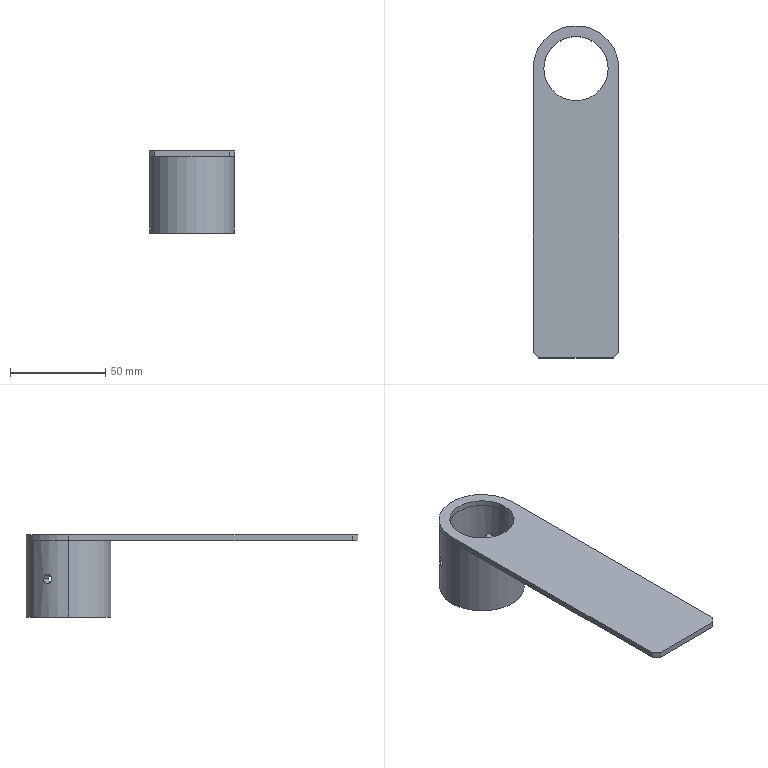Part | SolidWorks | features HoleWzd 3, 3DProfileFeature 1, Chamfer 1, Extrusion 1, ICE 1 | 2 solids | 20 faces | box 45 x 174.185 x 43 mm | volume 46480 mm3 | cylinder 11 | plane 9 | commonest cylinder face diameters 5 x4 33.7 x4 44.5 x2 45 x1
STEP:
#1=CARTESIAN_POINT('',(16.85,0.,20.));
#2=VERTEX_POINT('',#1);
#3=CARTESIAN_POINT('',(-16.85,0.,20.));
#4=VERTEX_POINT('',#3);
#5=CARTESIAN_POINT('',(0.,0.,20.));
#6=DIRECTION('',(0.,0.,-1.));
#7=DIRECTION('',(-1.,0.,0.));
#8=AXIS2_PLACEMENT_3D('',#5,#6,#7);
#9=CIRCLE('',#8,16.85);
#10=EDGE_CURVE('',#2,#4,#9,.T.);
#11=ORIENTED_EDGE('',*,*,#10,.T.);
#12=CARTESIAN_POINT('',(-16.85,0.,23.));
#13=VERTEX_POINT('',#12);
#14=CARTESIAN_POINT('',(-16.85,0.,23.));
#15=DIRECTION('',(0.,0.,1.));
#16=VECTOR('',#15,1000.);
#17=LINE('',#14,#16);
#18=EDGE_CURVE('',#4,#13,#17,.T.);
#19=ORIENTED_EDGE('',*,*,#18,.T.);
#20=CARTESIAN_POINT('',(16.85,0.,23.));
#21=VERTEX_POINT('',#20);
#22=CARTESIAN_POINT('',(0.,0.,23.));
#23=DIRECTION('',(0.,0.,1.));
#24=DIRECTION('',(1.,0.,0.));
#25=AXIS2_PLACEMENT_3D('',#22,#23,#24);
#26=CIRCLE('',#25,16.85);
#27=EDGE_CURVE('',#13,#21,#26,.T.);
#28=ORIENTED_EDGE('',*,*,#27,.T.);
#29=CARTESIAN_POINT('',(16.85,0.,23.));
#30=DIRECTION('',(0.,0.,1.));
#31=VECTOR('',#30,1000.);
#32=LINE('',#29,#31);
#33=EDGE_CURVE('',#2,#21,#32,.T.);
#34=ORIENTED_EDGE('',*,*,#33,.F.);
#35=EDGE_LOOP('',(#11,#19,#28,#34));
#36=FACE_OUTER_BOUND('',#35,.T.);
#37=CARTESIAN_POINT('',(0.,0.,23.));
#38=DIRECTION('',(0.,0.,1.));
#39=DIRECTION('',(1.,0.,0.));
#40=AXIS2_PLACEMENT_3D('',#37,#38,#39);
#41=CYLINDRICAL_SURFACE('',#40,16.85);
#42=ADVANCED_FACE('',(#36),#41,.F.);
#43=CARTESIAN_POINT('',(-22.5,0.,20.));
#44=VERTEX_POINT('',#43);
#45=CARTESIAN_POINT('',(22.5,0.,20.));
#46=VERTEX_POINT('',#45);
#47=CARTESIAN_POINT('',(0.,0.,20.));
#48=DIRECTION('',(0.,0.,-1.));
#49=DIRECTION('',(-1.,0.,0.));
#50=AXIS2_PLACEMENT_3D('',#47,#48,#49);
#51=CIRCLE('',#50,22.5);
#52=EDGE_CURVE('',#44,#46,#51,.T.);
#53=ORIENTED_EDGE('',*,*,#52,.F.);
#54=CARTESIAN_POINT('',(-22.5,0.,23.));
#55=VERTEX_POINT('',#54);
#56=CARTESIAN_POINT('',(-22.5,0.,23.));
#57=DIRECTION('',(0.,0.,-1.));
#58=VECTOR('',#57,1000.);
#59=LINE('',#56,#58);
#60=EDGE_CURVE('',#55,#44,#59,.T.);
#61=ORIENTED_EDGE('',*,*,#60,.F.);
#62=CARTESIAN_POINT('',(22.5,0.,23.));
#63=VERTEX_POINT('',#62);
#64=CARTESIAN_POINT('',(0.,0.,23.));
#65=DIRECTION('',(0.,0.,-1.));
#66=DIRECTION('',(-1.,0.,0.));
#67=AXIS2_PLACEMENT_3D('',#64,#65,#66);
#68=CIRCLE('',#67,22.5);
#69=EDGE_CURVE('',#55,#63,#68,.T.);
#70=ORIENTED_EDGE('',*,*,#69,.T.);
#71=CARTESIAN_POINT('',(22.5,0.,23.));
#72=DIRECTION('',(0.,0.,-1.));
#73=VECTOR('',#72,1000.);
#74=LINE('',#71,#73);
#75=EDGE_CURVE('',#63,#46,#74,.T.);
#76=ORIENTED_EDGE('',*,*,#75,.T.);
#77=EDGE_LOOP('',(#53,#61,#70,#76));
#78=FACE_OUTER_BOUND('',#77,.T.);
#79=CARTESIAN_POINT('',(0.,0.,23.));
#80=DIRECTION('',(0.,0.,-1.));
#81=DIRECTION('',(-1.,0.,0.));
#82=AXIS2_PLACEMENT_3D('',#79,#80,#81);
#83=CYLINDRICAL_SURFACE('',#82,22.5);
#84=ADVANCED_FACE('',(#78),#83,.T.);
#85=CARTESIAN_POINT('',(-22.5,-148.685,20.));
#86=VERTEX_POINT('',#85);
#87=CARTESIAN_POINT('',(-22.5,-151.685,20.));
#88=DIRECTION('',(0.,1.,0.));
#89=VECTOR('',#88,1000.);
#90=LINE('',#87,#89);
#91=EDGE_CURVE('',#86,#44,#90,.T.);
#92=ORIENTED_EDGE('',*,*,#91,.F.);
#93=CARTESIAN_POINT('',(-22.5,-148.685,23.));
#94=VERTEX_POINT('',#93);
#95=CARTESIAN_POINT('',(-22.5,-148.685,23.));
#96=DIRECTION('',(0.,0.,1.));
#97=VECTOR('',#96,1000.);
#98=LINE('',#95,#97);
#99=EDGE_CURVE('',#86,#94,#98,.T.);
#100=ORIENTED_EDGE('',*,*,#99,.T.);
#101=CARTESIAN_POINT('',(-22.5,-151.685,23.));
#102=DIRECTION('',(0.,1.,0.));
#103=VECTOR('',#102,1000.);
#104=LINE('',#101,#103);
#105=EDGE_CURVE('',#94,#55,#104,.T.);
#106=ORIENTED_EDGE('',*,*,#105,.T.);
#107=ORIENTED_EDGE('',*,*,#60,.T.);
#108=EDGE_LOOP('',(#92,#100,#106,#107));
#109=FACE_OUTER_BOUND('',#108,.T.);
#110=CARTESIAN_POINT('',(-22.5,-151.685,23.));
#111=DIRECTION('',(-1.,0.,0.));
#112=DIRECTION('',(0.,-1.,0.));
#113=AXIS2_PLACEMENT_3D('',#110,#111,#112);
#114=PLANE('',#113);
#115=ADVANCED_FACE('',(#109),#114,.T.);
#116=CARTESIAN_POINT('',(19.5,-151.685,23.));
#117=VERTEX_POINT('',#116);
#118=CARTESIAN_POINT('',(-19.5,-151.685,23.));
#119=VERTEX_POINT('',#118);
#120=CARTESIAN_POINT('',(22.5,-151.685,23.));
#121=DIRECTION('',(-1.,0.,0.));
#122=VECTOR('',#121,1000.);
#123=LINE('',#120,#122);
#124=EDGE_CURVE('',#117,#119,#123,.T.);
#125=ORIENTED_EDGE('',*,*,#124,.T.);
#126=CARTESIAN_POINT('',(-19.5,-151.685,20.));
#127=VERTEX_POINT('',#126);
#128=CARTESIAN_POINT('',(-19.5,-151.685,23.));
#129=DIRECTION('',(0.,0.,-1.));
#130=VECTOR('',#129,1000.);
#131=LINE('',#128,#130);
#132=EDGE_CURVE('',#119,#127,#131,.T.);
#133=ORIENTED_EDGE('',*,*,#132,.T.);
#134=CARTESIAN_POINT('',(19.5,-151.685,20.));
#135=VERTEX_POINT('',#134);
#136=CARTESIAN_POINT('',(22.5,-151.685,20.));
#137=DIRECTION('',(-1.,0.,0.));
#138=VECTOR('',#137,1000.);
#139=LINE('',#136,#138);
#140=EDGE_CURVE('',#135,#127,#139,.T.);
#141=ORIENTED_EDGE('',*,*,#140,.F.);
#142=CARTESIAN_POINT('',(19.5,-151.685,23.));
#143=DIRECTION('',(0.,0.,1.));
#144=VECTOR('',#143,1000.);
#145=LINE('',#142,#144);
#146=EDGE_CURVE('',#135,#117,#145,.T.);
#147=ORIENTED_EDGE('',*,*,#146,.T.);
#148=EDGE_LOOP('',(#125,#133,#141,#147));
#149=FACE_OUTER_BOUND('',#148,.T.);
#150=CARTESIAN_POINT('',(22.5,-151.685,23.));
#151=DIRECTION('',(0.,-1.,0.));
#152=DIRECTION('',(0.,0.,-1.));
#153=AXIS2_PLACEMENT_3D('',#150,#151,#152);
#154=PLANE('',#153);
#155=ADVANCED_FACE('',(#149),#154,.T.);
#156=CARTESIAN_POINT('',(22.5,-148.685,23.));
#157=VERTEX_POINT('',#156);
#158=CARTESIAN_POINT('',(22.5,0.,23.));
#159=DIRECTION('',(0.,-1.,0.));
#160=VECTOR('',#159,1000.);
#161=LINE('',#158,#160);
#162=EDGE_CURVE('',#63,#157,#161,.T.);
#163=ORIENTED_EDGE('',*,*,#162,.T.);
#164=CARTESIAN_POINT('',(22.5,-148.685,20.));
#165=VERTEX_POINT('',#164);
#166=CARTESIAN_POINT('',(22.5,-148.685,23.));
#167=DIRECTION('',(0.,0.,-1.));
#168=VECTOR('',#167,1000.);
#169=LINE('',#166,#168);
#170=EDGE_CURVE('',#157,#165,#169,.T.);
#171=ORIENTED_EDGE('',*,*,#170,.T.);
#172=CARTESIAN_POINT('',(22.5,0.,20.));
#173=DIRECTION('',(0.,-1.,0.));
#174=VECTOR('',#173,1000.);
#175=LINE('',#172,#174);
#176=EDGE_CURVE('',#46,#165,#175,.T.);
#177=ORIENTED_EDGE('',*,*,#176,.F.);
#178=ORIENTED_EDGE('',*,*,#75,.F.);
#179=EDGE_LOOP('',(#163,#171,#177,#178));
#180=FACE_OUTER_BOUND('',#179,.T.);
#181=CARTESIAN_POINT('',(22.5,0.,23.));
#182=DIRECTION('',(1.,0.,0.));
#183=DIRECTION('',(0.,1.,0.));
#184=AXIS2_PLACEMENT_3D('',#181,#182,#183);
#185=PLANE('',#184);
#186=ADVANCED_FACE('',(#180),#185,.T.);
#187=CARTESIAN_POINT('',(0.,0.,23.));
#188=DIRECTION('',(0.,0.,1.));
#189=DIRECTION('',(1.,0.,0.));
#190=AXIS2_PLACEMENT_3D('',#187,#188,#189);
#191=CIRCLE('',#190,16.85);
#192=EDGE_CURVE('',#21,#13,#191,.T.);
#193=ORIENTED_EDGE('',*,*,#192,.F.);
#194=ORIENTED_EDGE('',*,*,#27,.F.);
#195=EDGE_LOOP('',(#193,#194));
#196=FACE_BOUND('',#195,.T.);
#197=ORIENTED_EDGE('',*,*,#105,.F.);
#198=CARTESIAN_POINT('',(-19.5,-151.685,23.));
#199=DIRECTION('',(0.7071,-0.7071,0.));
#200=VECTOR('',#199,1000.);
#201=LINE('',#198,#200);
#202=EDGE_CURVE('',#94,#119,#201,.T.);
#203=ORIENTED_EDGE('',*,*,#202,.T.);
#204=ORIENTED_EDGE('',*,*,#124,.F.);
#205=CARTESIAN_POINT('',(22.5,-148.685,23.));
#206=DIRECTION('',(0.7071,0.7071,0.));
#207=VECTOR('',#206,1000.);
#208=LINE('',#205,#207);
#209=EDGE_CURVE('',#117,#157,#208,.T.);
#210=ORIENTED_EDGE('',*,*,#209,.T.);
#211=ORIENTED_EDGE('',*,*,#162,.F.);
#212=ORIENTED_EDGE('',*,*,#69,.F.);
#213=EDGE_LOOP('',(#197,#203,#204,#210,#211,#212));
#214=FACE_OUTER_BOUND('',#213,.T.);
#215=CARTESIAN_POINT('',(0.,0.,23.));
#216=DIRECTION('',(0.,0.,-1.));
#217=DIRECTION('',(-1.,0.,0.));
#218=AXIS2_PLACEMENT_3D('',#215,#216,#217);
#219=PLANE('',#218);
#220=ADVANCED_FACE('',(#196,#214),#219,.F.);
#221=ORIENTED_EDGE('',*,*,#10,.F.);
#222=CARTESIAN_POINT('',(0.,0.,20.));
#223=DIRECTION('',(0.,0.,-1.));
#224=DIRECTION('',(-1.,0.,0.));
#225=AXIS2_PLACEMENT_3D('',#222,#223,#224);
#226=CIRCLE('',#225,16.85);
#227=EDGE_CURVE('',#4,#2,#226,.T.);
#228=ORIENTED_EDGE('',*,*,#227,.F.);
#229=EDGE_LOOP('',(#221,#228));
#230=FACE_BOUND('',#229,.T.);
#231=ORIENTED_EDGE('',*,*,#140,.T.);
#232=CARTESIAN_POINT('',(-85.593,-85.593,20.));
#233=DIRECTION('',(-0.7071,0.7071,0.));
#234=VECTOR('',#233,1000.);
#235=LINE('',#232,#234);
#236=EDGE_CURVE('',#127,#86,#235,.T.);
#237=ORIENTED_EDGE('',*,*,#236,.T.);
#238=ORIENTED_EDGE('',*,*,#91,.T.);
#239=ORIENTED_EDGE('',*,*,#52,.T.);
#240=ORIENTED_EDGE('',*,*,#176,.T.);
#241=CARTESIAN_POINT('',(85.593,-85.593,20.));
#242=DIRECTION('',(-0.7071,-0.7071,0.));
#243=VECTOR('',#242,1000.);
#244=LINE('',#241,#243);
#245=EDGE_CURVE('',#165,#135,#244,.T.);
#246=ORIENTED_EDGE('',*,*,#245,.T.);
#247=EDGE_LOOP('',(#231,#237,#238,#239,#240,#246));
#248=FACE_OUTER_BOUND('',#247,.T.);
#249=CARTESIAN_POINT('',(0.,0.,20.));
#250=DIRECTION('',(0.,0.,-1.));
#251=DIRECTION('',(-1.,0.,0.));
#252=AXIS2_PLACEMENT_3D('',#249,#250,#251);
#253=PLANE('',#252);
#254=ADVANCED_FACE('',(#230,#248),#253,.T.);
#255=ORIENTED_EDGE('',*,*,#18,.F.);
#256=ORIENTED_EDGE('',*,*,#227,.T.);
#257=ORIENTED_EDGE('',*,*,#33,.T.);
#258=ORIENTED_EDGE('',*,*,#192,.T.);
#259=EDGE_LOOP('',(#255,#256,#257,#258));
#260=FACE_OUTER_BOUND('',#259,.T.);
#261=CARTESIAN_POINT('',(0.,0.,23.));
#262=DIRECTION('',(0.,0.,1.));
#263=DIRECTION('',(1.,0.,0.));
#264=AXIS2_PLACEMENT_3D('',#261,#262,#263);
#265=CYLINDRICAL_SURFACE('',#264,16.85);
#266=ADVANCED_FACE('',(#260),#265,.F.);
#267=ORIENTED_EDGE('',*,*,#202,.F.);
#268=ORIENTED_EDGE('',*,*,#99,.F.);
#269=ORIENTED_EDGE('',*,*,#236,.F.);
#270=ORIENTED_EDGE('',*,*,#132,.F.);
#271=EDGE_LOOP('',(#267,#268,#269,#270));
#272=FACE_OUTER_BOUND('',#271,.T.);
#273=CARTESIAN_POINT('',(-19.5,-151.685,23.));
#274=DIRECTION('',(0.7071,0.7071,0.));
#275=DIRECTION('',(0.,0.,-1.));
#276=AXIS2_PLACEMENT_3D('',#273,#274,#275);
#277=PLANE('',#276);
#278=ADVANCED_FACE('',(#272),#277,.F.);
#279=ORIENTED_EDGE('',*,*,#209,.F.);
#280=ORIENTED_EDGE('',*,*,#146,.F.);
#281=ORIENTED_EDGE('',*,*,#245,.F.);
#282=ORIENTED_EDGE('',*,*,#170,.F.);
#283=EDGE_LOOP('',(#279,#280,#281,#282));
#284=FACE_OUTER_BOUND('',#283,.T.);
#285=CARTESIAN_POINT('',(22.5,-148.685,23.));
#286=DIRECTION('',(-0.7071,0.7071,0.));
#287=DIRECTION('',(0.,0.,-1.));
#288=AXIS2_PLACEMENT_3D('',#285,#286,#287);
#289=PLANE('',#288);
#290=ADVANCED_FACE('',(#284),#289,.F.);
#291=CLOSED_SHELL('',(#42,#84,#115,#155,#186,#220,#254,#266,#278,#290));
#292=MANIFOLD_SOLID_BREP('',#291);
#293=CARTESIAN_POINT('',(17.897,13.22,0.));
#294=VERTEX_POINT('',#293);
#295=CARTESIAN_POINT('',(20.397,8.889,0.));
#296=VERTEX_POINT('',#295);
#297=CARTESIAN_POINT('',(17.897,13.22,0.));
#298=CARTESIAN_POINT('',(17.897,13.22,-0.1632));
#299=CARTESIAN_POINT('',(17.907,13.207,-0.3255));
#300=CARTESIAN_POINT('',(17.945,13.155,-0.6482));
#301=CARTESIAN_POINT('',(17.973,13.116,-0.8059));
#302=CARTESIAN_POINT('',(18.047,13.015,-1.107));
#303=CARTESIAN_POINT('',(18.092,12.951,-1.252));
#304=CARTESIAN_POINT('',(18.198,12.802,-1.525));
#305=CARTESIAN_POINT('',(18.258,12.717,-1.651));
#306=CARTESIAN_POINT('',(18.389,12.527,-1.882));
#307=CARTESIAN_POINT('',(18.461,12.42,-1.987));
#308=CARTESIAN_POINT('',(18.612,12.193,-2.169));
#309=CARTESIAN_POINT('',(18.69,12.073,-2.246));
#310=CARTESIAN_POINT('',(18.853,11.818,-2.372));
#311=CARTESIAN_POINT('',(18.937,11.683,-2.42));
#312=CARTESIAN_POINT('',(19.103,11.409,-2.484));
#313=CARTESIAN_POINT('',(19.186,11.27,-2.5));
#314=CARTESIAN_POINT('',(19.351,10.984,-2.5));
#315=CARTESIAN_POINT('',(19.43,10.842,-2.484));
#316=CARTESIAN_POINT('',(19.584,10.561,-2.421));
#317=CARTESIAN_POINT('',(19.659,10.421,-2.373));
#318=CARTESIAN_POINT('',(19.799,10.153,-2.247));
#319=CARTESIAN_POINT('',(19.864,10.024,-2.171));
#320=CARTESIAN_POINT('',(19.986,9.78,-1.99));
#321=CARTESIAN_POINT('',(20.042,9.664,-1.884));
#322=CARTESIAN_POINT('',(20.141,9.456,-1.654));
#323=CARTESIAN_POINT('',(20.185,9.361,-1.528));
#324=CARTESIAN_POINT('',(20.262,9.194,-1.255));
#325=CARTESIAN_POINT('',(20.294,9.123,-1.11));
#326=CARTESIAN_POINT('',(20.371,8.951,-0.659));
#327=CARTESIAN_POINT('',(20.397,8.889,-0.3306));
#328=CARTESIAN_POINT('',(20.397,8.889,0.));
#329=B_SPLINE_CURVE_WITH_KNOTS('',3,(#297,#298,#299,#300,#301,#302,#303,#304,#305,#306,#307,#308,#309,#310,#311,#312,#313,#314,#315,#316,#317,#318,#319,#320,#321,#322,#323,#324,#325,#326,#327,#328),.UNSPECIFIED.,.F.,.F.,(4,2,2,2,2,2,2,2,2,2,2,2,2,2,2,4),(0.007822,0.008311,0.0088,0.009289,0.009777,0.01027,0.01075,0.01124,0.01173,0.01222,0.01271,0.0132,0.01369,0.01418,0.01467,0.01564),.UNSPECIFIED.);
#330=EDGE_CURVE('',#294,#296,#329,.T.);
#331=ORIENTED_EDGE('',*,*,#330,.F.);
#332=CARTESIAN_POINT('',(13.181,10.497,0.));
#333=VERTEX_POINT('',#332);
#334=CARTESIAN_POINT('',(13.181,10.497,0.));
#335=DIRECTION('',(-0.866,-0.5,0.));
#336=VECTOR('',#335,1000.);
#337=LINE('',#334,#336);
#338=EDGE_CURVE('',#294,#333,#337,.T.);
#339=ORIENTED_EDGE('',*,*,#338,.T.);
#340=CARTESIAN_POINT('',(15.681,6.167,0.));
#341=VERTEX_POINT('',#340);
#342=CARTESIAN_POINT('',(15.681,6.167,0.));
#343=CARTESIAN_POINT('',(15.681,6.167,-0.1654));
#344=CARTESIAN_POINT('',(15.675,6.182,-0.328));
#345=CARTESIAN_POINT('',(15.651,6.242,-0.6479));
#346=CARTESIAN_POINT('',(15.633,6.287,-0.8068));
#347=CARTESIAN_POINT('',(15.586,6.404,-1.109));
#348=CARTESIAN_POINT('',(15.556,6.476,-1.253));
#349=CARTESIAN_POINT('',(15.485,6.645,-1.525));
#350=CARTESIAN_POINT('',(15.443,6.742,-1.653));
#351=CARTESIAN_POINT('',(15.349,6.954,-1.883));
#352=CARTESIAN_POINT('',(15.296,7.069,-1.987));
#353=CARTESIAN_POINT('',(15.179,7.317,-2.169));
#354=CARTESIAN_POINT('',(15.116,7.447,-2.247));
#355=CARTESIAN_POINT('',(14.98,7.717,-2.372));
#356=CARTESIAN_POINT('',(14.907,7.857,-2.42));
#357=CARTESIAN_POINT('',(14.754,8.141,-2.484));
#358=CARTESIAN_POINT('',(14.675,8.283,-2.5));
#359=CARTESIAN_POINT('',(14.511,8.566,-2.5));
#360=CARTESIAN_POINT('',(14.426,8.708,-2.484));
#361=CARTESIAN_POINT('',(14.258,8.981,-2.42));
#362=CARTESIAN_POINT('',(14.174,9.113,-2.372));
#363=CARTESIAN_POINT('',(14.008,9.367,-2.247));
#364=CARTESIAN_POINT('',(13.925,9.488,-2.169));
#365=CARTESIAN_POINT('',(13.771,9.711,-1.988));
#366=CARTESIAN_POINT('',(13.697,9.815,-1.884));
#367=CARTESIAN_POINT('',(13.559,10.004,-1.651));
#368=CARTESIAN_POINT('',(13.497,10.087,-1.525));
#369=CARTESIAN_POINT('',(13.387,10.233,-1.255));
#370=CARTESIAN_POINT('',(13.339,10.296,-1.108));
#371=CARTESIAN_POINT('',(13.261,10.396,-0.8059));
#372=CARTESIAN_POINT('',(13.232,10.433,-0.65));
#373=CARTESIAN_POINT('',(13.191,10.484,-0.3291));
#374=CARTESIAN_POINT('',(13.181,10.497,-0.1633));
#375=CARTESIAN_POINT('',(13.181,10.497,0.));
#376=B_SPLINE_CURVE_WITH_KNOTS('',3,(#342,#343,#344,#345,#346,#347,#348,#349,#350,#351,#352,#353,#354,#355,#356,#357,#358,#359,#360,#361,#362,#363,#364,#365,#366,#367,#368,#369,#370,#371,#372,#373,#374,#375),.UNSPECIFIED.,.F.,.F.,(4,2,2,2,2,2,2,2,2,2,2,2,2,2,2,2,4),(0.,0.0004892,0.0009784,0.001468,0.001957,0.002446,0.002935,0.003424,0.003913,0.004403,0.004892,0.005381,0.00587,0.006359,0.006849,0.007338,0.007827),.UNSPECIFIED.);
#377=EDGE_CURVE('',#341,#333,#376,.T.);
#378=ORIENTED_EDGE('',*,*,#377,.F.);
#379=CARTESIAN_POINT('',(15.681,6.167,0.));
#380=DIRECTION('',(-0.866,-0.5,0.));
#381=VECTOR('',#380,1000.);
#382=LINE('',#379,#381);
#383=EDGE_CURVE('',#296,#341,#382,.T.);
#384=ORIENTED_EDGE('',*,*,#383,.F.);
#385=EDGE_LOOP('',(#331,#339,#378,#384));
#386=FACE_OUTER_BOUND('',#385,.T.);
#387=CARTESIAN_POINT('',(14.431,8.332,0.));
#388=DIRECTION('',(-0.866,-0.5,0.));
#389=DIRECTION('',(0.5,-0.866,0.));
#390=AXIS2_PLACEMENT_3D('',#387,#388,#389);
#391=CYLINDRICAL_SURFACE('',#390,2.5);
#392=ADVANCED_FACE('',(#386),#391,.F.);
#393=CARTESIAN_POINT('',(-13.181,10.497,0.));
#394=VERTEX_POINT('',#393);
#395=CARTESIAN_POINT('',(-15.681,6.167,0.));
#396=VERTEX_POINT('',#395);
#397=CARTESIAN_POINT('',(-13.181,10.497,0.));
#398=CARTESIAN_POINT('',(-13.181,10.497,-0.3265));
#399=CARTESIAN_POINT('',(-13.223,10.445,-0.6558));
#400=CARTESIAN_POINT('',(-13.339,10.296,-1.107));
#401=CARTESIAN_POINT('',(-13.386,10.234,-1.253));
#402=CARTESIAN_POINT('',(-13.497,10.087,-1.526));
#403=CARTESIAN_POINT('',(-13.559,10.004,-1.651));
#404=CARTESIAN_POINT('',(-13.696,9.817,-1.882));
#405=CARTESIAN_POINT('',(-13.77,9.712,-1.987));
#406=CARTESIAN_POINT('',(-13.925,9.488,-2.169));
#407=CARTESIAN_POINT('',(-14.006,9.369,-2.246));
#408=CARTESIAN_POINT('',(-14.172,9.115,-2.371));
#409=CARTESIAN_POINT('',(-14.258,8.982,-2.42));
#410=CARTESIAN_POINT('',(-14.425,8.709,-2.484));
#411=CARTESIAN_POINT('',(-14.509,8.569,-2.5));
#412=CARTESIAN_POINT('',(-14.674,8.283,-2.5));
#413=CARTESIAN_POINT('',(-14.754,8.141,-2.484));
#414=CARTESIAN_POINT('',(-14.905,7.86,-2.421));
#415=CARTESIAN_POINT('',(-14.979,7.718,-2.372));
#416=CARTESIAN_POINT('',(-15.115,7.448,-2.247));
#417=CARTESIAN_POINT('',(-15.178,7.318,-2.171));
#418=CARTESIAN_POINT('',(-15.295,7.072,-1.989));
#419=CARTESIAN_POINT('',(-15.348,6.954,-1.884));
#420=CARTESIAN_POINT('',(-15.49,6.637,-1.539));
#421=CARTESIAN_POINT('',(-15.562,6.463,-1.261));
#422=CARTESIAN_POINT('',(-15.633,6.288,-0.8097));
#423=CARTESIAN_POINT('',(-15.651,6.243,-0.6518));
#424=CARTESIAN_POINT('',(-15.675,6.182,-0.3288));
#425=CARTESIAN_POINT('',(-15.681,6.167,-0.1654));
#426=CARTESIAN_POINT('',(-15.681,6.167,0.));
#427=B_SPLINE_CURVE_WITH_KNOTS('',3,(#397,#398,#399,#400,#401,#402,#403,#404,#405,#406,#407,#408,#409,#410,#411,#412,#413,#414,#415,#416,#417,#418,#419,#420,#421,#422,#423,#424,#425,#426),.UNSPECIFIED.,.F.,.F.,(4,2,2,2,2,2,2,2,2,2,2,2,2,2,4),(0.007827,0.008805,0.009294,0.009783,0.01027,0.01076,0.01125,0.01174,0.01223,0.01272,0.01321,0.0137,0.01467,0.01516,0.01565),.UNSPECIFIED.);
#428=EDGE_CURVE('',#394,#396,#427,.T.);
#429=ORIENTED_EDGE('',*,*,#428,.F.);
#430=CARTESIAN_POINT('',(-17.897,13.22,0.));
#431=VERTEX_POINT('',#430);
#432=CARTESIAN_POINT('',(-18.236,13.415,0.));
#433=DIRECTION('',(-0.866,0.5,0.));
#434=VECTOR('',#433,1000.);
#435=LINE('',#432,#434);
#436=EDGE_CURVE('',#394,#431,#435,.T.);
#437=ORIENTED_EDGE('',*,*,#436,.T.);
#438=CARTESIAN_POINT('',(-20.397,8.889,0.));
#439=VERTEX_POINT('',#438);
#440=CARTESIAN_POINT('',(-20.397,8.889,0.));
#441=CARTESIAN_POINT('',(-20.397,8.889,-0.1653));
#442=CARTESIAN_POINT('',(-20.391,8.904,-0.3279));
#443=CARTESIAN_POINT('',(-20.365,8.963,-0.6476));
#444=CARTESIAN_POINT('',(-20.345,9.007,-0.8064));
#445=CARTESIAN_POINT('',(-20.294,9.123,-1.109));
#446=CARTESIAN_POINT('',(-20.262,9.193,-1.253));
#447=CARTESIAN_POINT('',(-20.186,9.359,-1.524));
#448=CARTESIAN_POINT('',(-20.142,9.455,-1.653));
#449=CARTESIAN_POINT('',(-20.042,9.664,-1.883));
#450=CARTESIAN_POINT('',(-19.987,9.777,-1.987));
#451=CARTESIAN_POINT('',(-19.865,10.022,-2.17));
#452=CARTESIAN_POINT('',(-19.799,10.152,-2.247));
#453=CARTESIAN_POINT('',(-19.66,10.419,-2.372));
#454=CARTESIAN_POINT('',(-19.586,10.558,-2.42));
#455=CARTESIAN_POINT('',(-19.431,10.841,-2.484));
#456=CARTESIAN_POINT('',(-19.351,10.983,-2.5));
#457=CARTESIAN_POINT('',(-19.188,11.266,-2.5));
#458=CARTESIAN_POINT('',(-19.103,11.408,-2.484));
#459=CARTESIAN_POINT('',(-18.937,11.682,-2.42));
#460=CARTESIAN_POINT('',(-18.855,11.815,-2.373));
#461=CARTESIAN_POINT('',(-18.692,12.071,-2.247));
#462=CARTESIAN_POINT('',(-18.612,12.193,-2.169));
#463=CARTESIAN_POINT('',(-18.462,12.419,-1.988));
#464=CARTESIAN_POINT('',(-18.391,12.524,-1.885));
#465=CARTESIAN_POINT('',(-18.258,12.717,-1.651));
#466=CARTESIAN_POINT('',(-18.198,12.802,-1.525));
#467=CARTESIAN_POINT('',(-18.093,12.95,-1.254));
#468=CARTESIAN_POINT('',(-18.047,13.014,-1.108));
#469=CARTESIAN_POINT('',(-17.973,13.116,-0.8055));
#470=CARTESIAN_POINT('',(-17.945,13.155,-0.6497));
#471=CARTESIAN_POINT('',(-17.907,13.206,-0.329));
#472=CARTESIAN_POINT('',(-17.897,13.22,-0.1632));
#473=CARTESIAN_POINT('',(-17.897,13.22,0.));
#474=B_SPLINE_CURVE_WITH_KNOTS('',3,(#440,#441,#442,#443,#444,#445,#446,#447,#448,#449,#450,#451,#452,#453,#454,#455,#456,#457,#458,#459,#460,#461,#462,#463,#464,#465,#466,#467,#468,#469,#470,#471,#472,#473),.UNSPECIFIED.,.F.,.F.,(4,2,2,2,2,2,2,2,2,2,2,2,2,2,2,2,4),(0.,0.0004889,0.0009778,0.001467,0.001956,0.002444,0.002933,0.003422,0.003911,0.0044,0.004889,0.005378,0.005867,0.006356,0.006845,0.007333,0.007822),.UNSPECIFIED.);
#475=EDGE_CURVE('',#439,#431,#474,.T.);
#476=ORIENTED_EDGE('',*,*,#475,.F.);
#477=CARTESIAN_POINT('',(-20.736,9.085,0.));
#478=DIRECTION('',(-0.866,0.5,0.));
#479=VECTOR('',#478,1000.);
#480=LINE('',#477,#479);
#481=EDGE_CURVE('',#396,#439,#480,.T.);
#482=ORIENTED_EDGE('',*,*,#481,.F.);
#483=EDGE_LOOP('',(#429,#437,#476,#482));
#484=FACE_OUTER_BOUND('',#483,.T.);
#485=CARTESIAN_POINT('',(-19.486,11.25,0.));
#486=DIRECTION('',(-0.866,0.5,0.));
#487=DIRECTION('',(-0.5,-0.866,0.));
#488=AXIS2_PLACEMENT_3D('',#485,#486,#487);
#489=CYLINDRICAL_SURFACE('',#488,2.5);
#490=ADVANCED_FACE('',(#484),#489,.F.);
#491=CARTESIAN_POINT('',(-16.85,0.,-20.));
#492=VERTEX_POINT('',#491);
#493=CARTESIAN_POINT('',(16.85,0.,-20.));
#494=VERTEX_POINT('',#493);
#495=CARTESIAN_POINT('',(0.,0.,-20.));
#496=DIRECTION('',(0.,0.,1.));
#497=DIRECTION('',(1.,0.,0.));
#498=AXIS2_PLACEMENT_3D('',#495,#496,#497);
#499=CIRCLE('',#498,16.85);
#500=EDGE_CURVE('',#492,#494,#499,.T.);
#501=ORIENTED_EDGE('',*,*,#500,.F.);
#502=CARTESIAN_POINT('',(-16.85,0.,20.));
#503=VERTEX_POINT('',#502);
#504=CARTESIAN_POINT('',(-16.85,0.,23.));
#505=DIRECTION('',(0.,0.,1.));
#506=VECTOR('',#505,1000.);
#507=LINE('',#504,#506);
#508=EDGE_CURVE('',#492,#503,#507,.T.);
#509=ORIENTED_EDGE('',*,*,#508,.T.);
#510=CARTESIAN_POINT('',(16.85,0.,20.));
#511=VERTEX_POINT('',#510);
#512=CARTESIAN_POINT('',(0.,0.,20.));
#513=DIRECTION('',(0.,0.,-1.));
#514=DIRECTION('',(-1.,0.,0.));
#515=AXIS2_PLACEMENT_3D('',#512,#513,#514);
#516=CIRCLE('',#515,16.85);
#517=EDGE_CURVE('',#511,#503,#516,.T.);
#518=ORIENTED_EDGE('',*,*,#517,.F.);
#519=CARTESIAN_POINT('',(16.85,0.,23.));
#520=DIRECTION('',(0.,0.,1.));
#521=VECTOR('',#520,1000.);
#522=LINE('',#519,#521);
#523=EDGE_CURVE('',#494,#511,#522,.T.);
#524=ORIENTED_EDGE('',*,*,#523,.F.);
#525=EDGE_LOOP('',(#501,#509,#518,#524));
#526=FACE_OUTER_BOUND('',#525,.T.);
#527=CARTESIAN_POINT('',(0.,0.,23.));
#528=DIRECTION('',(0.,0.,1.));
#529=DIRECTION('',(1.,0.,0.));
#530=AXIS2_PLACEMENT_3D('',#527,#528,#529);
#531=CYLINDRICAL_SURFACE('',#530,16.85);
#532=ADVANCED_FACE('',(#526),#531,.F.);
#533=CARTESIAN_POINT('',(20.397,8.889,0.));
#534=CARTESIAN_POINT('',(20.397,8.889,0.1653));
#535=CARTESIAN_POINT('',(20.391,8.904,0.3279));
#536=CARTESIAN_POINT('',(20.365,8.963,0.6476));
#537=CARTESIAN_POINT('',(20.345,9.007,0.8064));
#538=CARTESIAN_POINT('',(20.294,9.123,1.109));
#539=CARTESIAN_POINT('',(20.262,9.193,1.253));
#540=CARTESIAN_POINT('',(20.186,9.359,1.524));
#541=CARTESIAN_POINT('',(20.142,9.455,1.653));
#542=CARTESIAN_POINT('',(20.042,9.664,1.883));
#543=CARTESIAN_POINT('',(19.987,9.777,1.987));
#544=CARTESIAN_POINT('',(19.865,10.022,2.17));
#545=CARTESIAN_POINT('',(19.799,10.152,2.247));
#546=CARTESIAN_POINT('',(19.66,10.419,2.372));
#547=CARTESIAN_POINT('',(19.586,10.558,2.42));
#548=CARTESIAN_POINT('',(19.431,10.841,2.484));
#549=CARTESIAN_POINT('',(19.351,10.983,2.5));
#550=CARTESIAN_POINT('',(19.188,11.266,2.5));
#551=CARTESIAN_POINT('',(19.103,11.408,2.484));
#552=CARTESIAN_POINT('',(18.937,11.682,2.42));
#553=CARTESIAN_POINT('',(18.855,11.815,2.373));
#554=CARTESIAN_POINT('',(18.692,12.071,2.247));
#555=CARTESIAN_POINT('',(18.612,12.193,2.169));
#556=CARTESIAN_POINT('',(18.462,12.419,1.988));
#557=CARTESIAN_POINT('',(18.391,12.524,1.885));
#558=CARTESIAN_POINT('',(18.258,12.717,1.651));
#559=CARTESIAN_POINT('',(18.198,12.802,1.525));
#560=CARTESIAN_POINT('',(18.093,12.95,1.254));
#561=CARTESIAN_POINT('',(18.047,13.014,1.108));
#562=CARTESIAN_POINT('',(17.973,13.116,0.8055));
#563=CARTESIAN_POINT('',(17.945,13.155,0.6497));
#564=CARTESIAN_POINT('',(17.907,13.206,0.329));
#565=CARTESIAN_POINT('',(17.897,13.22,0.1632));
#566=CARTESIAN_POINT('',(17.897,13.22,0.));
#567=B_SPLINE_CURVE_WITH_KNOTS('',3,(#533,#534,#535,#536,#537,#538,#539,#540,#541,#542,#543,#544,#545,#546,#547,#548,#549,#550,#551,#552,#553,#554,#555,#556,#557,#558,#559,#560,#561,#562,#563,#564,#565,#566),.UNSPECIFIED.,.F.,.F.,(4,2,2,2,2,2,2,2,2,2,2,2,2,2,2,2,4),(0.,0.0004889,0.0009778,0.001467,0.001956,0.002444,0.002933,0.003422,0.003911,0.0044,0.004889,0.005378,0.005867,0.006356,0.006845,0.007333,0.007822),.UNSPECIFIED.);
#568=EDGE_CURVE('',#296,#294,#567,.T.);
#569=ORIENTED_EDGE('',*,*,#568,.T.);
#570=ORIENTED_EDGE('',*,*,#330,.T.);
#571=EDGE_LOOP('',(#569,#570));
#572=FACE_BOUND('',#571,.T.);
#573=ORIENTED_EDGE('',*,*,#475,.T.);
#574=CARTESIAN_POINT('',(-17.897,13.22,0.));
#575=CARTESIAN_POINT('',(-17.897,13.22,0.1632));
#576=CARTESIAN_POINT('',(-17.907,13.207,0.3255));
#577=CARTESIAN_POINT('',(-17.945,13.155,0.6482));
#578=CARTESIAN_POINT('',(-17.973,13.116,0.8059));
#579=CARTESIAN_POINT('',(-18.047,13.015,1.107));
#580=CARTESIAN_POINT('',(-18.092,12.951,1.252));
#581=CARTESIAN_POINT('',(-18.198,12.802,1.525));
#582=CARTESIAN_POINT('',(-18.258,12.717,1.651));
#583=CARTESIAN_POINT('',(-18.389,12.527,1.882));
#584=CARTESIAN_POINT('',(-18.461,12.42,1.987));
#585=CARTESIAN_POINT('',(-18.612,12.193,2.169));
#586=CARTESIAN_POINT('',(-18.69,12.073,2.246));
#587=CARTESIAN_POINT('',(-18.853,11.818,2.372));
#588=CARTESIAN_POINT('',(-18.937,11.683,2.42));
#589=CARTESIAN_POINT('',(-19.103,11.409,2.484));
#590=CARTESIAN_POINT('',(-19.186,11.27,2.5));
#591=CARTESIAN_POINT('',(-19.351,10.984,2.5));
#592=CARTESIAN_POINT('',(-19.43,10.842,2.484));
#593=CARTESIAN_POINT('',(-19.584,10.561,2.421));
#594=CARTESIAN_POINT('',(-19.659,10.421,2.373));
#595=CARTESIAN_POINT('',(-19.799,10.153,2.247));
#596=CARTESIAN_POINT('',(-19.864,10.024,2.171));
#597=CARTESIAN_POINT('',(-19.986,9.78,1.99));
#598=CARTESIAN_POINT('',(-20.042,9.664,1.884));
#599=CARTESIAN_POINT('',(-20.141,9.456,1.654));
#600=CARTESIAN_POINT('',(-20.185,9.361,1.528));
#601=CARTESIAN_POINT('',(-20.262,9.194,1.255));
#602=CARTESIAN_POINT('',(-20.294,9.123,1.11));
#603=CARTESIAN_POINT('',(-20.371,8.951,0.659));
#604=CARTESIAN_POINT('',(-20.397,8.889,0.3306));
#605=CARTESIAN_POINT('',(-20.397,8.889,0.));
#606=B_SPLINE_CURVE_WITH_KNOTS('',3,(#574,#575,#576,#577,#578,#579,#580,#581,#582,#583,#584,#585,#586,#587,#588,#589,#590,#591,#592,#593,#594,#595,#596,#597,#598,#599,#600,#601,#602,#603,#604,#605),.UNSPECIFIED.,.F.,.F.,(4,2,2,2,2,2,2,2,2,2,2,2,2,2,2,4),(0.007822,0.008311,0.0088,0.009289,0.009777,0.01027,0.01075,0.01124,0.01173,0.01222,0.01271,0.0132,0.01369,0.01418,0.01467,0.01564),.UNSPECIFIED.);
#607=EDGE_CURVE('',#431,#439,#606,.T.);
#608=ORIENTED_EDGE('',*,*,#607,.T.);
#609=EDGE_LOOP('',(#573,#608));
#610=FACE_BOUND('',#609,.T.);
#611=CARTESIAN_POINT('',(-22.25,0.,-20.));
#612=VERTEX_POINT('',#611);
#613=CARTESIAN_POINT('',(22.25,0.,-20.));
#614=VERTEX_POINT('',#613);
#615=CARTESIAN_POINT('',(0.,0.,-20.));
#616=DIRECTION('',(0.,0.,-1.));
#617=DIRECTION('',(-1.,0.,0.));
#618=AXIS2_PLACEMENT_3D('',#615,#616,#617);
#619=CIRCLE('',#618,22.25);
#620=EDGE_CURVE('',#612,#614,#619,.T.);
#621=ORIENTED_EDGE('',*,*,#620,.F.);
#622=CARTESIAN_POINT('',(-22.25,0.,20.));
#623=VERTEX_POINT('',#622);
#624=CARTESIAN_POINT('',(-22.25,0.,-20.));
#625=DIRECTION('',(0.,0.,1.));
#626=VECTOR('',#625,1000.);
#627=LINE('',#624,#626);
#628=EDGE_CURVE('',#612,#623,#627,.T.);
#629=ORIENTED_EDGE('',*,*,#628,.T.);
#630=CARTESIAN_POINT('',(22.25,0.,20.));
#631=VERTEX_POINT('',#630);
#632=CARTESIAN_POINT('',(0.,0.,20.));
#633=DIRECTION('',(0.,0.,-1.));
#634=DIRECTION('',(-1.,0.,0.));
#635=AXIS2_PLACEMENT_3D('',#632,#633,#634);
#636=CIRCLE('',#635,22.25);
#637=EDGE_CURVE('',#623,#631,#636,.T.);
#638=ORIENTED_EDGE('',*,*,#637,.T.);
#639=CARTESIAN_POINT('',(22.25,0.,-20.));
#640=DIRECTION('',(0.,0.,1.));
#641=VECTOR('',#640,1000.);
#642=LINE('',#639,#641);
#643=EDGE_CURVE('',#614,#631,#642,.T.);
#644=ORIENTED_EDGE('',*,*,#643,.F.);
#645=EDGE_LOOP('',(#621,#629,#638,#644));
#646=FACE_OUTER_BOUND('',#645,.T.);
#647=CARTESIAN_POINT('',(0.,0.,-20.));
#648=DIRECTION('',(0.,0.,1.));
#649=DIRECTION('',(1.,0.,0.));
#650=AXIS2_PLACEMENT_3D('',#647,#648,#649);
#651=CYLINDRICAL_SURFACE('',#650,22.25);
#652=ADVANCED_FACE('',(#572,#610,#646),#651,.T.);
#653=ORIENTED_EDGE('',*,*,#628,.F.);
#654=CARTESIAN_POINT('',(0.,0.,-20.));
#655=DIRECTION('',(0.,0.,-1.));
#656=DIRECTION('',(-1.,0.,0.));
#657=AXIS2_PLACEMENT_3D('',#654,#655,#656);
#658=CIRCLE('',#657,22.25);
#659=EDGE_CURVE('',#614,#612,#658,.T.);
#660=ORIENTED_EDGE('',*,*,#659,.F.);
#661=ORIENTED_EDGE('',*,*,#643,.T.);
#662=CARTESIAN_POINT('',(0.,0.,20.));
#663=DIRECTION('',(0.,0.,-1.));
#664=DIRECTION('',(-1.,0.,0.));
#665=AXIS2_PLACEMENT_3D('',#662,#663,#664);
#666=CIRCLE('',#665,22.25);
#667=EDGE_CURVE('',#631,#623,#666,.T.);
#668=ORIENTED_EDGE('',*,*,#667,.T.);
#669=EDGE_LOOP('',(#653,#660,#661,#668));
#670=FACE_OUTER_BOUND('',#669,.T.);
#671=CARTESIAN_POINT('',(0.,0.,-20.));
#672=DIRECTION('',(0.,0.,1.));
#673=DIRECTION('',(1.,0.,0.));
#674=AXIS2_PLACEMENT_3D('',#671,#672,#673);
#675=CYLINDRICAL_SURFACE('',#674,22.25);
#676=ADVANCED_FACE('',(#670),#675,.T.);
#677=CARTESIAN_POINT('',(0.,0.,-20.));
#678=DIRECTION('',(0.,0.,1.));
#679=DIRECTION('',(1.,0.,0.));
#680=AXIS2_PLACEMENT_3D('',#677,#678,#679);
#681=CIRCLE('',#680,16.85);
#682=EDGE_CURVE('',#494,#492,#681,.T.);
#683=ORIENTED_EDGE('',*,*,#682,.T.);
#684=ORIENTED_EDGE('',*,*,#500,.T.);
#685=EDGE_LOOP('',(#683,#684));
#686=FACE_BOUND('',#685,.T.);
#687=ORIENTED_EDGE('',*,*,#659,.T.);
#688=ORIENTED_EDGE('',*,*,#620,.T.);
#689=EDGE_LOOP('',(#687,#688));
#690=FACE_OUTER_BOUND('',#689,.T.);
#691=CARTESIAN_POINT('',(0.,0.,-20.));
#692=DIRECTION('',(0.,0.,-1.));
#693=DIRECTION('',(-1.,0.,0.));
#694=AXIS2_PLACEMENT_3D('',#691,#692,#693);
#695=PLANE('',#694);
#696=ADVANCED_FACE('',(#686,#690),#695,.T.);
#697=ORIENTED_EDGE('',*,*,#517,.T.);
#698=CARTESIAN_POINT('',(0.,0.,20.));
#699=DIRECTION('',(0.,0.,-1.));
#700=DIRECTION('',(-1.,0.,0.));
#701=AXIS2_PLACEMENT_3D('',#698,#699,#700);
#702=CIRCLE('',#701,16.85);
#703=EDGE_CURVE('',#503,#511,#702,.T.);
#704=ORIENTED_EDGE('',*,*,#703,.T.);
#705=EDGE_LOOP('',(#697,#704));
#706=FACE_BOUND('',#705,.T.);
#707=ORIENTED_EDGE('',*,*,#667,.F.);
#708=ORIENTED_EDGE('',*,*,#637,.F.);
#709=EDGE_LOOP('',(#707,#708));
#710=FACE_OUTER_BOUND('',#709,.T.);
#711=CARTESIAN_POINT('',(0.,0.,20.));
#712=DIRECTION('',(0.,0.,-1.));
#713=DIRECTION('',(-1.,0.,0.));
#714=AXIS2_PLACEMENT_3D('',#711,#712,#713);
#715=PLANE('',#714);
#716=ADVANCED_FACE('',(#706,#710),#715,.F.);
#717=ORIENTED_EDGE('',*,*,#508,.F.);
#718=ORIENTED_EDGE('',*,*,#682,.F.);
#719=ORIENTED_EDGE('',*,*,#523,.T.);
#720=ORIENTED_EDGE('',*,*,#703,.F.);
#721=EDGE_LOOP('',(#717,#718,#719,#720));
#722=FACE_OUTER_BOUND('',#721,.T.);
#723=ORIENTED_EDGE('',*,*,#377,.T.);
#724=CARTESIAN_POINT('',(13.181,10.497,0.));
#725=CARTESIAN_POINT('',(13.181,10.497,0.3265));
#726=CARTESIAN_POINT('',(13.223,10.445,0.6558));
#727=CARTESIAN_POINT('',(13.339,10.296,1.107));
#728=CARTESIAN_POINT('',(13.386,10.234,1.253));
#729=CARTESIAN_POINT('',(13.497,10.087,1.526));
#730=CARTESIAN_POINT('',(13.559,10.004,1.651));
#731=CARTESIAN_POINT('',(13.696,9.817,1.882));
#732=CARTESIAN_POINT('',(13.77,9.712,1.987));
#733=CARTESIAN_POINT('',(13.925,9.488,2.169));
#734=CARTESIAN_POINT('',(14.006,9.369,2.246));
#735=CARTESIAN_POINT('',(14.172,9.115,2.371));
#736=CARTESIAN_POINT('',(14.258,8.982,2.42));
#737=CARTESIAN_POINT('',(14.425,8.709,2.484));
#738=CARTESIAN_POINT('',(14.509,8.569,2.5));
#739=CARTESIAN_POINT('',(14.674,8.283,2.5));
#740=CARTESIAN_POINT('',(14.754,8.141,2.484));
#741=CARTESIAN_POINT('',(14.905,7.86,2.421));
#742=CARTESIAN_POINT('',(14.979,7.718,2.372));
#743=CARTESIAN_POINT('',(15.115,7.448,2.247));
#744=CARTESIAN_POINT('',(15.178,7.318,2.171));
#745=CARTESIAN_POINT('',(15.295,7.072,1.989));
#746=CARTESIAN_POINT('',(15.348,6.954,1.884));
#747=CARTESIAN_POINT('',(15.49,6.637,1.539));
#748=CARTESIAN_POINT('',(15.562,6.463,1.261));
#749=CARTESIAN_POINT('',(15.633,6.288,0.8097));
#750=CARTESIAN_POINT('',(15.651,6.243,0.6518));
#751=CARTESIAN_POINT('',(15.675,6.182,0.3288));
#752=CARTESIAN_POINT('',(15.681,6.167,0.1654));
#753=CARTESIAN_POINT('',(15.681,6.167,0.));
#754=B_SPLINE_CURVE_WITH_KNOTS('',3,(#724,#725,#726,#727,#728,#729,#730,#731,#732,#733,#734,#735,#736,#737,#738,#739,#740,#741,#742,#743,#744,#745,#746,#747,#748,#749,#750,#751,#752,#753),.UNSPECIFIED.,.F.,.F.,(4,2,2,2,2,2,2,2,2,2,2,2,2,2,4),(0.007827,0.008805,0.009294,0.009783,0.01027,0.01076,0.01125,0.01174,0.01223,0.01272,0.01321,0.0137,0.01467,0.01516,0.01565),.UNSPECIFIED.);
#755=EDGE_CURVE('',#333,#341,#754,.T.);
#756=ORIENTED_EDGE('',*,*,#755,.T.);
#757=EDGE_LOOP('',(#723,#756));
#758=FACE_BOUND('',#757,.T.);
#759=CARTESIAN_POINT('',(-15.681,6.167,0.));
#760=CARTESIAN_POINT('',(-15.681,6.167,0.1654));
#761=CARTESIAN_POINT('',(-15.675,6.182,0.328));
#762=CARTESIAN_POINT('',(-15.651,6.242,0.6479));
#763=CARTESIAN_POINT('',(-15.633,6.287,0.8068));
#764=CARTESIAN_POINT('',(-15.586,6.404,1.109));
#765=CARTESIAN_POINT('',(-15.556,6.476,1.253));
#766=CARTESIAN_POINT('',(-15.485,6.645,1.525));
#767=CARTESIAN_POINT('',(-15.443,6.742,1.653));
#768=CARTESIAN_POINT('',(-15.349,6.954,1.883));
#769=CARTESIAN_POINT('',(-15.296,7.069,1.987));
#770=CARTESIAN_POINT('',(-15.179,7.317,2.169));
#771=CARTESIAN_POINT('',(-15.116,7.447,2.247));
#772=CARTESIAN_POINT('',(-14.98,7.717,2.372));
#773=CARTESIAN_POINT('',(-14.907,7.857,2.42));
#774=CARTESIAN_POINT('',(-14.754,8.141,2.484));
#775=CARTESIAN_POINT('',(-14.675,8.283,2.5));
#776=CARTESIAN_POINT('',(-14.511,8.566,2.5));
#777=CARTESIAN_POINT('',(-14.426,8.708,2.484));
#778=CARTESIAN_POINT('',(-14.258,8.981,2.42));
#779=CARTESIAN_POINT('',(-14.174,9.113,2.372));
#780=CARTESIAN_POINT('',(-14.008,9.367,2.247));
#781=CARTESIAN_POINT('',(-13.925,9.488,2.169));
#782=CARTESIAN_POINT('',(-13.771,9.711,1.988));
#783=CARTESIAN_POINT('',(-13.697,9.815,1.884));
#784=CARTESIAN_POINT('',(-13.559,10.004,1.651));
#785=CARTESIAN_POINT('',(-13.497,10.087,1.525));
#786=CARTESIAN_POINT('',(-13.387,10.233,1.255));
#787=CARTESIAN_POINT('',(-13.339,10.296,1.108));
#788=CARTESIAN_POINT('',(-13.261,10.396,0.8059));
#789=CARTESIAN_POINT('',(-13.232,10.433,0.65));
#790=CARTESIAN_POINT('',(-13.191,10.484,0.3291));
#791=CARTESIAN_POINT('',(-13.181,10.497,0.1633));
#792=CARTESIAN_POINT('',(-13.181,10.497,0.));
#793=B_SPLINE_CURVE_WITH_KNOTS('',3,(#759,#760,#761,#762,#763,#764,#765,#766,#767,#768,#769,#770,#771,#772,#773,#774,#775,#776,#777,#778,#779,#780,#781,#782,#783,#784,#785,#786,#787,#788,#789,#790,#791,#792),.UNSPECIFIED.,.F.,.F.,(4,2,2,2,2,2,2,2,2,2,2,2,2,2,2,2,4),(0.,0.0004892,0.0009784,0.001468,0.001957,0.002446,0.002935,0.003424,0.003913,0.004403,0.004892,0.005381,0.00587,0.006359,0.006849,0.007338,0.007827),.UNSPECIFIED.);
#794=EDGE_CURVE('',#396,#394,#793,.T.);
#795=ORIENTED_EDGE('',*,*,#794,.T.);
#796=ORIENTED_EDGE('',*,*,#428,.T.);
#797=EDGE_LOOP('',(#795,#796));
#798=FACE_BOUND('',#797,.T.);
#799=CARTESIAN_POINT('',(0.,0.,23.));
#800=DIRECTION('',(0.,0.,1.));
#801=DIRECTION('',(1.,0.,0.));
#802=AXIS2_PLACEMENT_3D('',#799,#800,#801);
#803=CYLINDRICAL_SURFACE('',#802,16.85);
#804=ADVANCED_FACE('',(#722,#758,#798),#803,.F.);
#805=ORIENTED_EDGE('',*,*,#436,.F.);
#806=ORIENTED_EDGE('',*,*,#794,.F.);
#807=ORIENTED_EDGE('',*,*,#481,.T.);
#808=ORIENTED_EDGE('',*,*,#607,.F.);
#809=EDGE_LOOP('',(#805,#806,#807,#808));
#810=FACE_OUTER_BOUND('',#809,.T.);
#811=CARTESIAN_POINT('',(-19.486,11.25,0.));
#812=DIRECTION('',(-0.866,0.5,0.));
#813=DIRECTION('',(-0.5,-0.866,0.));
#814=AXIS2_PLACEMENT_3D('',#811,#812,#813);
#815=CYLINDRICAL_SURFACE('',#814,2.5);
#816=ADVANCED_FACE('',(#810),#815,.F.);
#817=ORIENTED_EDGE('',*,*,#338,.F.);
#818=ORIENTED_EDGE('',*,*,#568,.F.);
#819=ORIENTED_EDGE('',*,*,#383,.T.);
#820=ORIENTED_EDGE('',*,*,#755,.F.);
#821=EDGE_LOOP('',(#817,#818,#819,#820));
#822=FACE_OUTER_BOUND('',#821,.T.);
#823=CARTESIAN_POINT('',(14.431,8.332,0.));
#824=DIRECTION('',(-0.866,-0.5,0.));
#825=DIRECTION('',(0.5,-0.866,0.));
#826=AXIS2_PLACEMENT_3D('',#823,#824,#825);
#827=CYLINDRICAL_SURFACE('',#826,2.5);
#828=ADVANCED_FACE('',(#822),#827,.F.);
#829=CLOSED_SHELL('',(#392,#490,#532,#652,#676,#696,#716,#804,#816,#828));
#830=MANIFOLD_SOLID_BREP('',#829);
#831=CARTESIAN_POINT('',(0.,0.,0.));
#832=DIRECTION('',(0.,0.,1.));
#833=DIRECTION('',(1.,0.,0.));
#834=AXIS2_PLACEMENT_3D('',#831,#832,#833);
#835=(LENGTH_UNIT()NAMED_UNIT(*)SI_UNIT(.MILLI.,.METRE.));
#836=UNCERTAINTY_MEASURE_WITH_UNIT(LENGTH_MEASURE(0.00001),#835,'','');
#837=(NAMED_UNIT(*)PLANE_ANGLE_UNIT()SI_UNIT($,.RADIAN.));
#838=(NAMED_UNIT(*)SI_UNIT($,.STERADIAN.)SOLID_ANGLE_UNIT());
#839=(GEOMETRIC_REPRESENTATION_CONTEXT(3)GLOBAL_UNCERTAINTY_ASSIGNED_CONTEXT((#836))GLOBAL_UNIT_ASSIGNED_CONTEXT((#835,#837,#838))REPRESENTATION_CONTEXT('',''));
#840=ADVANCED_BREP_SHAPE_REPRESENTATION('',(#292,#830,#834),#839);